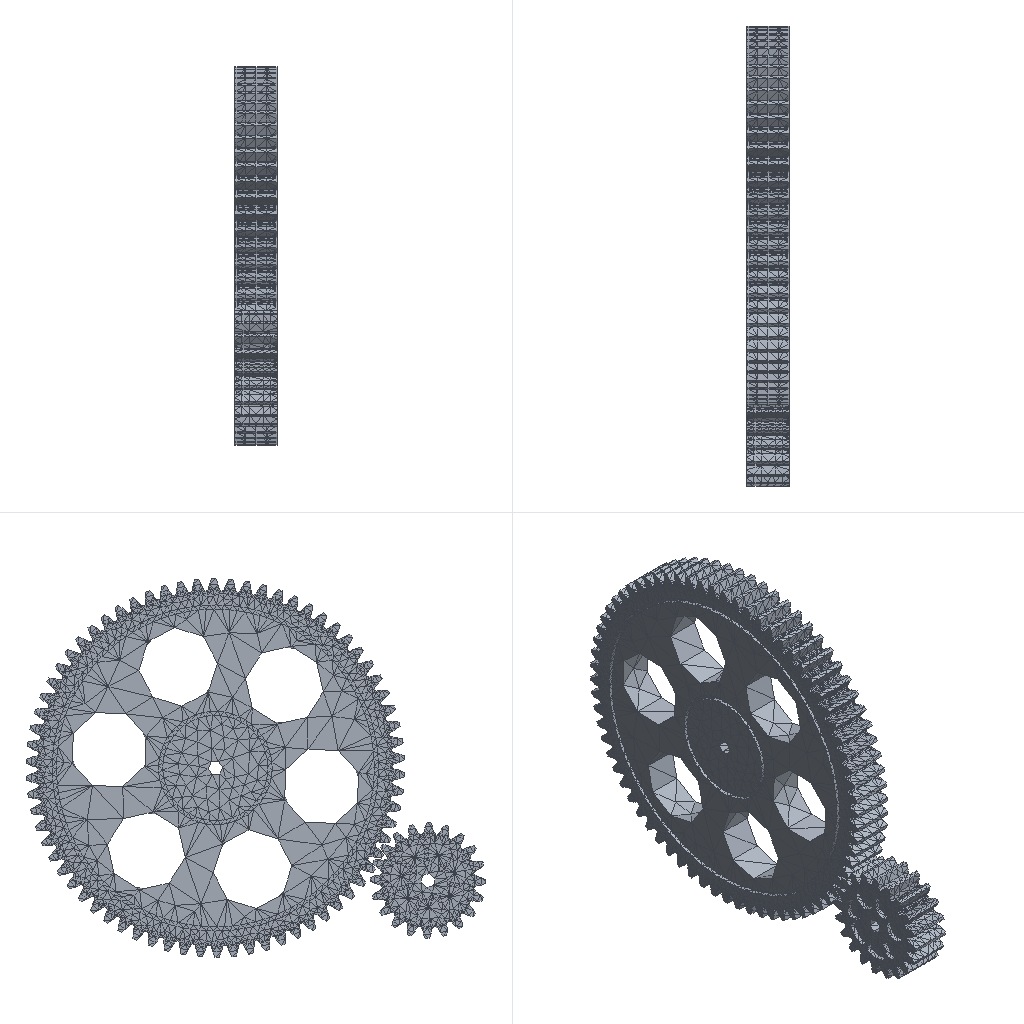Simulation study
Set-up summary:
category,name,step,type,value,unit,region
solver,ansys_mapdl
solver,version,,,22.1
units,MPA,,stated
analysis,deck,,transient,transient
load_step,requested,,,1
analysis,nlgeom,,,True
mesh,nodes,,,53924
mesh,elements,,,29590
element_type,ANSYS 187 (type 1),,solid,23679
element_type,ANSYS 187 (type 2),,solid,5534
element_type,ANSYS 174 (type 3),,contact,108
element_type,ANSYS 170 (type 4),,target,108
element_type,ANSYS 174 (type 5),,contact,161
element_type,ANSYS 170 (type 6),,target,0
load,load commands in deck,,count,3
bc,support commands in deck,,count,1
named_set,_FIXEDSU,,component
material,1,,in results
material,2,,in results
check,setup vs results,,match,results also hold 1 node(s) and 1 element(s) the deck makes with ['EN']; those were not compared
Ansys APDL input file, long lists of numbers shortened:
/batch
/config,noeldb,1     ! force off writing results to database
*get,_wallstrt,active,,time,wall
! ANSYS input file written by Workbench version 2022 R1
! File used for geometry attach: F:\ansys（分析文件汇总)\瞬态齿轮有限元分析\装配体2^冲床总装配.STEP
/title,wbnew--__ (B5)
! ****** Begin Custom Load Command Snippet ******
/COM, ACT Extensions:
/COM,     LSDYNA, 2021.1
/COM,
! ****** End   Custom Load Command Snippet ******
*DIM,_wb_ProjectScratch_dir,string,248
_wb_ProjectScratch_dir(1) = 'C:\Users\Administrator\AppData\Local\Temp\WB_Administrator_26156_2\_ProjectScratch\Scr01F2\'
*DIM,_wb_SolverFiles_dir,string,248
_wb_SolverFiles_dir(1) = 'C:\Users\Administrator\AppData\Local\Temp\WB_Administrator_26156_2\wbnew_files\dp0\SYS\MECH\'
*DIM,_wb_userfiles_dir,string,248
_wb_userfiles_dir(1) = 'C:\Users\Administrator\AppData\Local\Temp\WB_Administrator_26156_2\wbnew_files\user_files\'
/com,--- Data in consistent NMM units. See Solving Units in the help system for more information.
/units,MPA
/nopr
/wb,file,start              !  signify a WB generated input file
/prep7
! Turn off shape checking because checks already performed inside WB mesher.
! See help system for more information.
SHPP,OFF,,NOWARN
/nolist
etcon,set             ! allow ANSYS to choose best KEYOP's for 180x elements, resets any applicable keyopt to MAPDL defaults
/com,*********** Nodes for the whole assembly ***********
nblock,3,,59315
(1i9,3e20.9e3)
        1    -5.889179435E+01    -1.875993906E+01     1.185023106E+02
! (53922 more lines like these left out)
-1
/com,*********** Nodes for all Remote Points ***********
nblock,3
(1i9,3e20.9e3)
    53924    -5.589567727E+01    -1.312721965E+01     1.232014297E+02
-1
/wb,elem,start            !  set before creation of elements
/com,*********** Elements for Body 1 "_____.sldasm-Part-21|____1" ***********
et,1,187
eblock,19,solid,,23679
(19i9)
        1        1        1        1        0        0        0        0       10        0     5535    13819    17555    14902    15317    38367    43798    38364    38365
! (47357 more lines like these left out)
-1
/com,*********** Elements for Body 2 "_____.sldasm-Part-39|____1" ***********
et,2,187
eblock,19,solid,,5534
(19i9)
        2        2        2        2        0        0        0        0       10        0        1     1374     1528     1731     1698     9254    10060     9260     9259
! (11067 more lines like these left out)
-1
/wb,elem,end               !  done creating elements
/com,*********** Send User Defined Coordinate System(s) ***********
csys,0
toffst,273.15,  ! Temperature offset from absolute zero
/com,*********** Set Reference Temperature ***********
tref,22.
/wb,mat,start              !  starting to send materials
/com,*********** Send Materials ***********
Temperature = 'TEMP' ! Temperature
MP,DENS,1,7.85e-09,	! tonne mm^-3
MP,ALPX,1,1.2e-05,	! C^-1
MP,C,1,434000000,	! mm^2 s^-2 C^-1
MP,KXX,1,60.5,	! tonne mm s^-3 C^-1
MP,RSVX,1,0.00017,	! ohm mm
MP,EX,1,200000,	! tonne s^-2 mm^-1
MP,NUXY,1,0.3,
MP,MURX,1,10000,
Temperature = 'TEMP' ! Temperature
MP,DENS,2,7.85e-09,	! tonne mm^-3
MP,ALPX,2,1.2e-05,	! C^-1
MP,C,2,434000000,	! mm^2 s^-2 C^-1
MP,KXX,2,60.5,	! tonne mm s^-3 C^-1
MP,RSVX,2,0.00017,	! ohm mm
MP,EX,2,200000,	! tonne s^-2 mm^-1
MP,NUXY,2,0.3,
MP,MURX,2,10000,
/wb,mat,end                !  done sending materials
!************************* Model Summary ********************
!_____.sldasm-Part-21|____1,	45钢,	matid,	1
!_____.sldasm-Part-39|____1,	45钢,	matid,	2
!************************* End Model Summary ********************
! get the diagonal of the bounding box. Needed later for other things
*get,_xmin,node,,mnloc,x
*get,_ymin,node,,mnloc,y
*get,_zmin,node,,mnloc,z
*get,_xmax,node,,mxloc,x
*get,_ymax,node,,mxloc,y
*get,_zmax,node,,mxloc,z
_ASMDIAG=(_xmax-_xmin)*(_xmax-_xmin)+(_ymax-_ymin)*(_ymax-_ymin)+(_zmax-_zmin)*(_zmax-_zmin)
_ASMDIAG=SQRT(_ASMDIAG)
/wb,contact,start          !  starting to send contact
/com,*********** Create Contact "接触区域" ***********
/com,            Real Constant Set For Above Contact Is 4 & 3
*set,tid,4
*set,cid,3
r,tid
r,cid
et,tid,170
et,cid,174
eblock,10,,,56
(15i9)
    43059        4        4        4        0    11814    13764    14385    14385    26531    38104    14385    26533
! (55 more lines like these left out)
-1
eblock,10,,,56
(15i9)
    43115        3        3        3        0    11814    13764    14385    14385    26531    38104    14385    26533
! (55 more lines like these left out)
-1
eblock,10,,,52
(15i9)
    43171        3        4        3        0      454      944      819      819     4486     6745      819     4485
! (51 more lines like these left out)
-1
eblock,10,,,52
(15i9)
    43223        4        3        4        0      454      944      819      819     4486     6745      819     4485
! (51 more lines like these left out)
-1
keyo,cid,8,2               ! auto create asymmetric contact (from Program Controlled setting)
keyo,cid,10,0              ! adjust contact stiffness each NR iteration (from Program Controlled setting)
keyo,cid,12,5              ! bonded always
keyo,cid,18,1              ! small sliding turned on by application
keyo,cid,2,0               ! augmented Lagrange (from Program Controlled setting)
keyo,cid,4,0               ! on Gauss point (from Program Controlled setting)
keyo,cid,9,1               ! ignore initial gaps/penetration
keyo,cid,7,0               ! No Prediction
rmod,tid,3,10.      ! FKN
rmod,tid,5,0.       ! ICONT
rmod,tid,6,0.       ! PINB
rmod,tid,10,0.      ! CNOF
rmod,tid,12,0.      ! FKT
rmod,tid,36,29      ! WB DSID
rmod,cid,3,10.      ! FKN
rmod,cid,5,0.       ! ICONT
rmod,cid,6,0.       ! PINB
rmod,cid,10,0.      ! CNOF
rmod,cid,12,0.      ! FKT
rmod,cid,36,29      ! WB DSID
nsel,all
esel,all
/wb,contact,end            !  done creating contacts
/golist
/wb,load,start             !  starting to send loads
/com,*********** Fixed Supports ***********
CMBLOCK,_FIXEDSU,NODE,      252
(8i10)
         9        10        11        12        13        14        15        16
! (31 more lines like these left out)
cmsel,s,_FIXEDSU
d,all,all
nsel,all
/com,*********** Create Remote Point "内部远程点" ***********
! -------- Remote Point Used by "力矩" --------
*set,tid,6
*set,cid,5
et,cid,174
et,tid,170
keyo,tid,2,1               ! Don't fix the pilot node
keyo,tid,4,0               ! Activate all DOF's due to large deformation
keyo,cid,12,5              ! Bonded Contact
keyo,cid,4,1               ! Deformable RBE3 style load
keyo,cid,2,2               ! MPC style contact
eblock,10,,,161
(15i9)
    43275        5        5        5        0      463      938      821      821     4534     6752      821     4533
! (160 more lines like these left out)
-1
*set,_npilot,53924
_npilot42=_npilot
type,tid
mat ,cid
real,cid
tshape,pilo
en,43436,_npilot
tshape
/com,*********** Construct Moment Using Remote Attachment ***********
/gst,on,on
fini
*get,_numnode,node,0,count
*get,_numelem,elem,0,count
*get, _MAXELEMNUM, elem, 0, NUM, MAX
*get, _MAXNODENUM, node, 0, NUM, MAX
*get, _MAXELEMTYPE, etyp, 0, NUM, MAX
*get, _MAXREALCONST, real, 0, NUM, MAX
/go
/wb,load,end               !  done creating loads
/com,--- Number of total nodes = %_numnode%
/com,--- Number of contact elements = 377
/com,--- Number of spring elements = 0
/com,--- Number of bearing elements = 0
/com,--- Number of solid elements = 29213
/com,--- Number of condensed parts = 0
/com,--- Number of total elements = %_numelem%
*get,_wallbsol,active,,time,wall
/com,****************************************************************************
/com,*************************    SOLUTION       ********************************
/com,****************************************************************************
/solu
antype,4                   ! transient analysis
nlgeom,on                  ! Turn on Large Deformation Effects
kbc,1                      ! stepped BC's
_thickRatio=  1     ! Ratio of thick parts in the model
eqsl,pcg,1e-8,,,,,,1
cntr,print,1               ! print out contact info and also make no initial contact an error
dmpoption,emat,no             ! Don't combine emat file for DANSYS
dmpoption,esav,no             ! Don't combine esav file for DANSYS
trnopt,full,,,,,hht        ! HHT time integration method
tintp, mosp			! Choose transient integration settings for moderate speed application
nldiag,cont,iter           ! print out contact info each equilibrium iteration
rescontrol,define,last,last,,dele	   ! Program Controlled
/com,****************************************************
/com,******************* SOLVE FOR LS 1 OF 1 ****************
nsel,s,node,,53924
f,all,mx,5000.
f,all,my,0.
f,all,mz,0.
nsel,all
/nopr
/gopr
autots,on                   ! User turned on automatic time stepping
deltim,1,1,1,OFF
time,1.
timint,on                  ! Turn on time integration effects
outres,erase
outres,all,none
outres,nsol,all,
outres,rsol,all
outres,eangl,all
outres,etmp,all
outres,veng,all
outres,strs,all,
outres,epel,all,
outres,eppl,all,
outres,cont,all,
outres,v,all,
outres,a,all,
! *********** WB SOLVE COMMAND ***********
! check interactive state
*get,ANSINTER_,active,,int
*if,ANSINTER_,ne,0,then
/eof
*endif
solve
/com *************** Write FE CONNECTORS *********
CEWRITE,file,ce,,INTE
/com,****************************************************
/com,*************** FINISHED SOLVE FOR LS 1 *************
*get,_wallasol,active,,time,wall
/nopr
*get,_numnode,node,0,count
*get,_numelem,elem,0,count
*get, _MAXELEMNUM, elem, 0, NUM, MAX
*get, _MAXNODENUM, node, 0, NUM, MAX,,,INTERNAL
*get, _MAXELEMTYPE, etyp, 0, NUM, MAX
*get, _MAXREALCONST, real, 0, NUM, MAX
/gopr
*get,_PCGITER,active,,solu,cgiter
/post1
xmlo,ENCODING,ISO-8859-1
xmlo,parm
/xml,parm,xml
fini
/gopr
*get,_walldone,active,,time,wall
_preptime=(_wallbsol-_wallstrt)*3600
_solvtime=(_wallasol-_wallbsol)*3600
_posttime=(_walldone-_wallasol)*3600
_totaltim=(_walldone-_wallstrt)*3600
*get,_dlbratio,active,0,solu,dlbr
*get,_combtime,active,0,solu,comb
*get,_ssmode,active,0,solu,ssmm
*get,_ndofs,active,0,solu,ndof
*get,_sol_end_time,active,0,set,time
*if,_sol_end_time,eq,1.,then
/fclean				!clean distributed files
*endif
/com,--- Total number of nodes = %_numnode%
/com,--- Total number of elements = %_numelem%
/com,--- Element load balance ratio = %_dlbratio%
/com,--- Time to combine distributed files = %_combtime%
/com,--- Sparse memory mode = %_ssmode%
/com,--- Number of DOF = %_ndofs%
/wb,file,end               ! done with WB generated input
Results summary:
result,analysis,,,static
result,last_loadstep,,,1
result,primary field,,,displacement
result,reaction total,1,FX,-0.0,N
result,reaction total,1,FY,-5e-06,N
result,reaction total,1,FZ,7e-06,N
result,mass,,,0.000167,"NMM: mm, ton, N, s, mV, mA, degC"